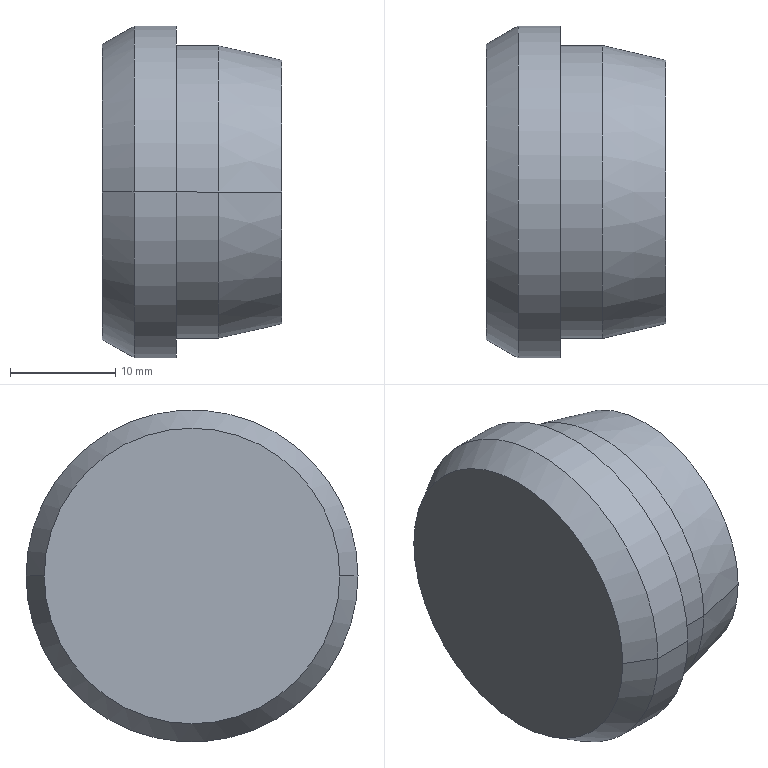Part | STEP file | DCV-000-041 | 1 solid | 11 faces | box 17 x 31.5 x 31.5 mm | volume 10923 mm3 | cone 4 | cylinder 4 | plane 3 | commonest cylinder face diameters 27.8 x2 31.5 x2
STEP:
#1=CARTESIAN_POINT('',(0.,0.,0.));
#2=DIRECTION('',(0.,0.,1.));
#3=DIRECTION('',(1.,0.,0.));
#4=AXIS2_PLACEMENT_3D('',#1,#2,#3);
#5=CARTESIAN_POINT('',(0.,14.018,0.));
#6=VERTEX_POINT('',#5);
#7=CARTESIAN_POINT('',(0.,-14.018,0.));
#8=VERTEX_POINT('',#7);
#9=CARTESIAN_POINT('',(0.,0.,0.));
#10=DIRECTION('',(1.,0.,0.));
#11=DIRECTION('',(0.,0.,-1.));
#12=AXIS2_PLACEMENT_3D('',#9,#10,#11);
#13=CIRCLE('',#12,14.018);
#14=CARTESIAN_POINT('',(1.5,0.,0.));
#15=DIRECTION('',(1.,0.,0.));
#16=DIRECTION('',(0.,1.,0.));
#17=AXIS2_PLACEMENT_3D('',#14,#15,#16);
#18=CONICAL_SURFACE('',#17,14.884,0.5236);
#19=CARTESIAN_POINT('',(-1.571,-1.5));
#20=DIRECTION('',(1.,0.));
#21=VECTOR('',#20,1.);
#22=LINE('',#19,#21);
#23=(GEOMETRIC_REPRESENTATION_CONTEXT(2)PARAMETRIC_REPRESENTATION_CONTEXT()REPRESENTATION_CONTEXT('',''));
#24=DEFINITIONAL_REPRESENTATION('',(#22),#23);
#25=PCURVE('',#18,#24);
#26=CARTESIAN_POINT('',(0.,14.018,0.));
#27=DIRECTION('',(-1.,0.,0.));
#28=DIRECTION('',(0.,0.,1.));
#29=AXIS2_PLACEMENT_3D('',#26,#27,#28);
#30=PLANE('',#29);
#31=CARTESIAN_POINT('',(-14.018,-14.018));
#32=CARTESIAN_POINT('',(-14.018,10.262));
#33=CARTESIAN_POINT('',(7.009,-1.878));
#34=CARTESIAN_POINT('',(28.036,-14.018));
#35=CARTESIAN_POINT('',(7.009,-26.158));
#36=CARTESIAN_POINT('',(-14.018,-38.298));
#37=CARTESIAN_POINT('',(-14.018,-14.018));
#38=(BOUNDED_CURVE()B_SPLINE_CURVE(2,(#31,#32,#33,#34,#35,#36,#37),.UNSPECIFIED.,.T.,.F.)B_SPLINE_CURVE_WITH_KNOTS((1,2,2,2,2,1),(-2.094,0.,2.094,4.189,6.283,8.378),.UNSPECIFIED.)CURVE()GEOMETRIC_REPRESENTATION_ITEM()RATIONAL_B_SPLINE_CURVE((1.,0.5,1.,0.5,1.,0.5,1.))REPRESENTATION_ITEM(''));
#39=(GEOMETRIC_REPRESENTATION_CONTEXT(2)PARAMETRIC_REPRESENTATION_CONTEXT()REPRESENTATION_CONTEXT('',''));
#40=DEFINITIONAL_REPRESENTATION('',(#38),#39);
#41=PCURVE('',#30,#40);
#42=SURFACE_CURVE('',#13,(#25,#41),.PCURVE_S1.);
#43=EDGE_CURVE('',#6,#8,#42,.T.);
#44=ORIENTED_EDGE('',*,*,#43,.T.);
#45=CARTESIAN_POINT('',(3.,-15.75,0.));
#46=VERTEX_POINT('',#45);
#47=CARTESIAN_POINT('',(1.5,-14.884,0.));
#48=DIRECTION('',(0.866,-0.5,0.));
#49=VECTOR('',#48,1.);
#50=LINE('',#47,#49);
#51=CARTESIAN_POINT('',(3.142,0.));
#52=DIRECTION('',(0.,1.));
#53=VECTOR('',#52,1.);
#54=LINE('',#51,#53);
#55=(GEOMETRIC_REPRESENTATION_CONTEXT(2)PARAMETRIC_REPRESENTATION_CONTEXT()REPRESENTATION_CONTEXT('',''));
#56=DEFINITIONAL_REPRESENTATION('',(#54),#55);
#57=PCURVE('',#18,#56);
#58=CARTESIAN_POINT('',(1.5,0.,0.));
#59=DIRECTION('',(1.,0.,0.));
#60=DIRECTION('',(0.,1.,0.));
#61=AXIS2_PLACEMENT_3D('',#58,#59,#60);
#62=CONICAL_SURFACE('',#61,14.884,0.5236);
#63=CARTESIAN_POINT('',(3.142,0.));
#64=DIRECTION('',(0.,1.));
#65=VECTOR('',#64,1.);
#66=LINE('',#63,#65);
#67=(GEOMETRIC_REPRESENTATION_CONTEXT(2)PARAMETRIC_REPRESENTATION_CONTEXT()REPRESENTATION_CONTEXT('',''));
#68=DEFINITIONAL_REPRESENTATION('',(#66),#67);
#69=PCURVE('',#62,#68);
#70=SURFACE_CURVE('',#50,(#57,#69),.PCURVE_S1.);
#71=EDGE_CURVE('',#8,#46,#70,.T.);
#72=ORIENTED_EDGE('',*,*,#71,.T.);
#73=CARTESIAN_POINT('',(3.,15.75,0.));
#74=VERTEX_POINT('',#73);
#75=CARTESIAN_POINT('',(3.,0.,0.));
#76=DIRECTION('',(1.,0.,0.));
#77=DIRECTION('',(0.,0.,-1.));
#78=AXIS2_PLACEMENT_3D('',#75,#76,#77);
#79=CIRCLE('',#78,15.75);
#80=CARTESIAN_POINT('',(-1.571,1.5));
#81=DIRECTION('',(1.,0.));
#82=VECTOR('',#81,1.);
#83=LINE('',#80,#82);
#84=(GEOMETRIC_REPRESENTATION_CONTEXT(2)PARAMETRIC_REPRESENTATION_CONTEXT()REPRESENTATION_CONTEXT('',''));
#85=DEFINITIONAL_REPRESENTATION('',(#83),#84);
#86=PCURVE('',#18,#85);
#87=CARTESIAN_POINT('',(5.,0.,0.));
#88=DIRECTION('',(1.,0.,0.));
#89=DIRECTION('',(0.,1.,0.));
#90=AXIS2_PLACEMENT_3D('',#87,#88,#89);
#91=CYLINDRICAL_SURFACE('',#90,15.75);
#92=CARTESIAN_POINT('',(-1.571,-2.));
#93=DIRECTION('',(1.,0.));
#94=VECTOR('',#93,1.);
#95=LINE('',#92,#94);
#96=(GEOMETRIC_REPRESENTATION_CONTEXT(2)PARAMETRIC_REPRESENTATION_CONTEXT()REPRESENTATION_CONTEXT('',''));
#97=DEFINITIONAL_REPRESENTATION('',(#95),#96);
#98=PCURVE('',#91,#97);
#99=SURFACE_CURVE('',#79,(#86,#98),.PCURVE_S1.);
#100=EDGE_CURVE('',#74,#46,#99,.T.);
#101=ORIENTED_EDGE('',*,*,#100,.F.);
#102=CARTESIAN_POINT('',(1.5,14.884,0.));
#103=DIRECTION('',(0.866,0.5,0.));
#104=VECTOR('',#103,1.);
#105=LINE('',#102,#104);
#106=CARTESIAN_POINT('',(0.,0.));
#107=DIRECTION('',(0.,1.));
#108=VECTOR('',#107,1.);
#109=LINE('',#106,#108);
#110=(GEOMETRIC_REPRESENTATION_CONTEXT(2)PARAMETRIC_REPRESENTATION_CONTEXT()REPRESENTATION_CONTEXT('',''));
#111=DEFINITIONAL_REPRESENTATION('',(#109),#110);
#112=PCURVE('',#18,#111);
#113=CARTESIAN_POINT('',(6.283,0.));
#114=DIRECTION('',(0.,1.));
#115=VECTOR('',#114,1.);
#116=LINE('',#113,#115);
#117=(GEOMETRIC_REPRESENTATION_CONTEXT(2)PARAMETRIC_REPRESENTATION_CONTEXT()REPRESENTATION_CONTEXT('',''));
#118=DEFINITIONAL_REPRESENTATION('',(#116),#117);
#119=PCURVE('',#62,#118);
#120=SURFACE_CURVE('',#105,(#112,#119),.PCURVE_S1.);
#121=EDGE_CURVE('',#6,#74,#120,.T.);
#122=ORIENTED_EDGE('',*,*,#121,.F.);
#123=EDGE_LOOP('',(#44,#72,#101,#122));
#124=FACE_BOUND('',#123,.T.);
#125=ADVANCED_FACE('',(#124),#18,.T.);
#126=ORIENTED_EDGE('',*,*,#100,.T.);
#127=CARTESIAN_POINT('',(7.,-15.75,0.));
#128=VERTEX_POINT('',#127);
#129=CARTESIAN_POINT('',(5.,-15.75,0.));
#130=DIRECTION('',(1.,0.,0.));
#131=VECTOR('',#130,1.);
#132=LINE('',#129,#131);
#133=CARTESIAN_POINT('',(3.142,0.));
#134=DIRECTION('',(0.,1.));
#135=VECTOR('',#134,1.);
#136=LINE('',#133,#135);
#137=(GEOMETRIC_REPRESENTATION_CONTEXT(2)PARAMETRIC_REPRESENTATION_CONTEXT()REPRESENTATION_CONTEXT('',''));
#138=DEFINITIONAL_REPRESENTATION('',(#136),#137);
#139=PCURVE('',#91,#138);
#140=CARTESIAN_POINT('',(5.,0.,0.));
#141=DIRECTION('',(1.,0.,0.));
#142=DIRECTION('',(0.,1.,0.));
#143=AXIS2_PLACEMENT_3D('',#140,#141,#142);
#144=CYLINDRICAL_SURFACE('',#143,15.75);
#145=CARTESIAN_POINT('',(3.142,0.));
#146=DIRECTION('',(0.,1.));
#147=VECTOR('',#146,1.);
#148=LINE('',#145,#147);
#149=(GEOMETRIC_REPRESENTATION_CONTEXT(2)PARAMETRIC_REPRESENTATION_CONTEXT()REPRESENTATION_CONTEXT('',''));
#150=DEFINITIONAL_REPRESENTATION('',(#148),#149);
#151=PCURVE('',#144,#150);
#152=SURFACE_CURVE('',#132,(#139,#151),.PCURVE_S1.);
#153=EDGE_CURVE('',#46,#128,#152,.T.);
#154=ORIENTED_EDGE('',*,*,#153,.T.);
#155=CARTESIAN_POINT('',(7.,15.75,0.));
#156=VERTEX_POINT('',#155);
#157=CARTESIAN_POINT('',(7.,0.,0.));
#158=DIRECTION('',(1.,0.,0.));
#159=DIRECTION('',(0.,0.,-1.));
#160=AXIS2_PLACEMENT_3D('',#157,#158,#159);
#161=CIRCLE('',#160,15.75);
#162=CARTESIAN_POINT('',(-1.571,2.));
#163=DIRECTION('',(1.,0.));
#164=VECTOR('',#163,1.);
#165=LINE('',#162,#164);
#166=(GEOMETRIC_REPRESENTATION_CONTEXT(2)PARAMETRIC_REPRESENTATION_CONTEXT()REPRESENTATION_CONTEXT('',''));
#167=DEFINITIONAL_REPRESENTATION('',(#165),#166);
#168=PCURVE('',#91,#167);
#169=CARTESIAN_POINT('',(7.,13.9,0.));
#170=DIRECTION('',(1.,0.,0.));
#171=DIRECTION('',(0.,-1.,0.));
#172=AXIS2_PLACEMENT_3D('',#169,#170,#171);
#173=PLANE('',#172);
#174=CARTESIAN_POINT('',(13.9,0.));
#175=DIRECTION('',(0.,1.));
#176=AXIS2_PLACEMENT_2D('',#174,#175);
#177=CIRCLE('',#176,15.75);
#178=(GEOMETRIC_REPRESENTATION_CONTEXT(2)PARAMETRIC_REPRESENTATION_CONTEXT()REPRESENTATION_CONTEXT('',''));
#179=DEFINITIONAL_REPRESENTATION('',(#177),#178);
#180=PCURVE('',#173,#179);
#181=SURFACE_CURVE('',#161,(#168,#180),.PCURVE_S1.);
#182=EDGE_CURVE('',#156,#128,#181,.T.);
#183=ORIENTED_EDGE('',*,*,#182,.F.);
#184=CARTESIAN_POINT('',(5.,15.75,0.));
#185=DIRECTION('',(1.,0.,0.));
#186=VECTOR('',#185,1.);
#187=LINE('',#184,#186);
#188=CARTESIAN_POINT('',(0.,0.));
#189=DIRECTION('',(0.,1.));
#190=VECTOR('',#189,1.);
#191=LINE('',#188,#190);
#192=(GEOMETRIC_REPRESENTATION_CONTEXT(2)PARAMETRIC_REPRESENTATION_CONTEXT()REPRESENTATION_CONTEXT('',''));
#193=DEFINITIONAL_REPRESENTATION('',(#191),#192);
#194=PCURVE('',#91,#193);
#195=CARTESIAN_POINT('',(6.283,0.));
#196=DIRECTION('',(0.,1.));
#197=VECTOR('',#196,1.);
#198=LINE('',#195,#197);
#199=(GEOMETRIC_REPRESENTATION_CONTEXT(2)PARAMETRIC_REPRESENTATION_CONTEXT()REPRESENTATION_CONTEXT('',''));
#200=DEFINITIONAL_REPRESENTATION('',(#198),#199);
#201=PCURVE('',#144,#200);
#202=SURFACE_CURVE('',#187,(#194,#201),.PCURVE_S1.);
#203=EDGE_CURVE('',#74,#156,#202,.T.);
#204=ORIENTED_EDGE('',*,*,#203,.F.);
#205=EDGE_LOOP('',(#126,#154,#183,#204));
#206=FACE_BOUND('',#205,.T.);
#207=ADVANCED_FACE('',(#206),#91,.T.);
#208=CARTESIAN_POINT('',(7.,13.9,0.));
#209=VERTEX_POINT('',#208);
#210=CARTESIAN_POINT('',(7.,-13.9,0.));
#211=VERTEX_POINT('',#210);
#212=CARTESIAN_POINT('',(7.,0.,0.));
#213=DIRECTION('',(1.,0.,0.));
#214=DIRECTION('',(0.,0.,-1.));
#215=AXIS2_PLACEMENT_3D('',#212,#213,#214);
#216=CIRCLE('',#215,13.9);
#217=CARTESIAN_POINT('',(9.,0.,0.));
#218=DIRECTION('',(1.,0.,0.));
#219=DIRECTION('',(0.,1.,0.));
#220=AXIS2_PLACEMENT_3D('',#217,#218,#219);
#221=CYLINDRICAL_SURFACE('',#220,13.9);
#222=CARTESIAN_POINT('',(-1.571,-2.));
#223=DIRECTION('',(1.,0.));
#224=VECTOR('',#223,1.);
#225=LINE('',#222,#224);
#226=(GEOMETRIC_REPRESENTATION_CONTEXT(2)PARAMETRIC_REPRESENTATION_CONTEXT()REPRESENTATION_CONTEXT('',''));
#227=DEFINITIONAL_REPRESENTATION('',(#225),#226);
#228=PCURVE('',#221,#227);
#229=CARTESIAN_POINT('',(13.9,0.));
#230=DIRECTION('',(0.,1.));
#231=AXIS2_PLACEMENT_2D('',#229,#230);
#232=CIRCLE('',#231,13.9);
#233=(GEOMETRIC_REPRESENTATION_CONTEXT(2)PARAMETRIC_REPRESENTATION_CONTEXT()REPRESENTATION_CONTEXT('',''));
#234=DEFINITIONAL_REPRESENTATION('',(#232),#233);
#235=PCURVE('',#173,#234);
#236=SURFACE_CURVE('',#216,(#228,#235),.PCURVE_S1.);
#237=EDGE_CURVE('',#209,#211,#236,.T.);
#238=ORIENTED_EDGE('',*,*,#237,.T.);
#239=CARTESIAN_POINT('',(11.,-13.9,0.));
#240=VERTEX_POINT('',#239);
#241=CARTESIAN_POINT('',(9.,-13.9,0.));
#242=DIRECTION('',(1.,0.,0.));
#243=VECTOR('',#242,1.);
#244=LINE('',#241,#243);
#245=CARTESIAN_POINT('',(3.142,0.));
#246=DIRECTION('',(0.,1.));
#247=VECTOR('',#246,1.);
#248=LINE('',#245,#247);
#249=(GEOMETRIC_REPRESENTATION_CONTEXT(2)PARAMETRIC_REPRESENTATION_CONTEXT()REPRESENTATION_CONTEXT('',''));
#250=DEFINITIONAL_REPRESENTATION('',(#248),#249);
#251=PCURVE('',#221,#250);
#252=CARTESIAN_POINT('',(9.,0.,0.));
#253=DIRECTION('',(1.,0.,0.));
#254=DIRECTION('',(0.,1.,0.));
#255=AXIS2_PLACEMENT_3D('',#252,#253,#254);
#256=CYLINDRICAL_SURFACE('',#255,13.9);
#257=CARTESIAN_POINT('',(3.142,0.));
#258=DIRECTION('',(0.,1.));
#259=VECTOR('',#258,1.);
#260=LINE('',#257,#259);
#261=(GEOMETRIC_REPRESENTATION_CONTEXT(2)PARAMETRIC_REPRESENTATION_CONTEXT()REPRESENTATION_CONTEXT('',''));
#262=DEFINITIONAL_REPRESENTATION('',(#260),#261);
#263=PCURVE('',#256,#262);
#264=SURFACE_CURVE('',#244,(#251,#263),.PCURVE_S1.);
#265=EDGE_CURVE('',#211,#240,#264,.T.);
#266=ORIENTED_EDGE('',*,*,#265,.T.);
#267=CARTESIAN_POINT('',(11.,13.9,0.));
#268=VERTEX_POINT('',#267);
#269=CARTESIAN_POINT('',(11.,0.,0.));
#270=DIRECTION('',(1.,0.,0.));
#271=DIRECTION('',(0.,0.,-1.));
#272=AXIS2_PLACEMENT_3D('',#269,#270,#271);
#273=CIRCLE('',#272,13.9);
#274=CARTESIAN_POINT('',(-1.571,2.));
#275=DIRECTION('',(1.,0.));
#276=VECTOR('',#275,1.);
#277=LINE('',#274,#276);
#278=(GEOMETRIC_REPRESENTATION_CONTEXT(2)PARAMETRIC_REPRESENTATION_CONTEXT()REPRESENTATION_CONTEXT('',''));
#279=DEFINITIONAL_REPRESENTATION('',(#277),#278);
#280=PCURVE('',#221,#279);
#281=CARTESIAN_POINT('',(14.,0.,0.));
#282=DIRECTION('',(-1.,0.,0.));
#283=DIRECTION('',(0.,1.,0.));
#284=AXIS2_PLACEMENT_3D('',#281,#282,#283);
#285=CONICAL_SURFACE('',#284,13.2,0.2292);
#286=CARTESIAN_POINT('',(7.854,3.));
#287=DIRECTION('',(-1.,0.));
#288=VECTOR('',#287,1.);
#289=LINE('',#286,#288);
#290=(GEOMETRIC_REPRESENTATION_CONTEXT(2)PARAMETRIC_REPRESENTATION_CONTEXT()REPRESENTATION_CONTEXT('',''));
#291=DEFINITIONAL_REPRESENTATION('',(#289),#290);
#292=PCURVE('',#285,#291);
#293=SURFACE_CURVE('',#273,(#280,#292),.PCURVE_S1.);
#294=EDGE_CURVE('',#268,#240,#293,.T.);
#295=ORIENTED_EDGE('',*,*,#294,.F.);
#296=CARTESIAN_POINT('',(9.,13.9,0.));
#297=DIRECTION('',(1.,0.,0.));
#298=VECTOR('',#297,1.);
#299=LINE('',#296,#298);
#300=CARTESIAN_POINT('',(0.,0.));
#301=DIRECTION('',(0.,1.));
#302=VECTOR('',#301,1.);
#303=LINE('',#300,#302);
#304=(GEOMETRIC_REPRESENTATION_CONTEXT(2)PARAMETRIC_REPRESENTATION_CONTEXT()REPRESENTATION_CONTEXT('',''));
#305=DEFINITIONAL_REPRESENTATION('',(#303),#304);
#306=PCURVE('',#221,#305);
#307=CARTESIAN_POINT('',(6.283,0.));
#308=DIRECTION('',(0.,1.));
#309=VECTOR('',#308,1.);
#310=LINE('',#307,#309);
#311=(GEOMETRIC_REPRESENTATION_CONTEXT(2)PARAMETRIC_REPRESENTATION_CONTEXT()REPRESENTATION_CONTEXT('',''));
#312=DEFINITIONAL_REPRESENTATION('',(#310),#311);
#313=PCURVE('',#256,#312);
#314=SURFACE_CURVE('',#299,(#306,#313),.PCURVE_S1.);
#315=EDGE_CURVE('',#209,#268,#314,.T.);
#316=ORIENTED_EDGE('',*,*,#315,.F.);
#317=EDGE_LOOP('',(#238,#266,#295,#316));
#318=FACE_BOUND('',#317,.T.);
#319=ADVANCED_FACE('',(#318),#221,.T.);
#320=CARTESIAN_POINT('',(17.,-12.5,0.));
#321=VERTEX_POINT('',#320);
#322=CARTESIAN_POINT('',(17.,12.5,0.));
#323=VERTEX_POINT('',#322);
#324=CARTESIAN_POINT('',(17.,0.,0.));
#325=DIRECTION('',(1.,0.,0.));
#326=DIRECTION('',(0.,0.,-1.));
#327=AXIS2_PLACEMENT_3D('',#324,#325,#326);
#328=CIRCLE('',#327,12.5);
#329=CARTESIAN_POINT('',(14.,0.,0.));
#330=DIRECTION('',(-1.,0.,0.));
#331=DIRECTION('',(0.,1.,0.));
#332=AXIS2_PLACEMENT_3D('',#329,#330,#331);
#333=CONICAL_SURFACE('',#332,13.2,0.2292);
#334=CARTESIAN_POINT('',(7.854,-3.));
#335=DIRECTION('',(-1.,0.));
#336=VECTOR('',#335,1.);
#337=LINE('',#334,#336);
#338=(GEOMETRIC_REPRESENTATION_CONTEXT(2)PARAMETRIC_REPRESENTATION_CONTEXT()REPRESENTATION_CONTEXT('',''));
#339=DEFINITIONAL_REPRESENTATION('',(#337),#338);
#340=PCURVE('',#333,#339);
#341=CARTESIAN_POINT('',(17.,0.,0.));
#342=DIRECTION('',(1.,0.,0.));
#343=DIRECTION('',(0.,-1.,0.));
#344=AXIS2_PLACEMENT_3D('',#341,#342,#343);
#345=PLANE('',#344);
#346=CARTESIAN_POINT('',(0.,0.));
#347=DIRECTION('',(0.,1.));
#348=AXIS2_PLACEMENT_2D('',#346,#347);
#349=CIRCLE('',#348,12.5);
#350=(GEOMETRIC_REPRESENTATION_CONTEXT(2)PARAMETRIC_REPRESENTATION_CONTEXT()REPRESENTATION_CONTEXT('',''));
#351=DEFINITIONAL_REPRESENTATION('',(#349),#350);
#352=PCURVE('',#345,#351);
#353=SURFACE_CURVE('',#328,(#340,#352),.PCURVE_S1.);
#354=EDGE_CURVE('',#321,#323,#353,.T.);
#355=ORIENTED_EDGE('',*,*,#354,.F.);
#356=CARTESIAN_POINT('',(14.,-13.2,0.));
#357=DIRECTION('',(-0.9738,-0.2272,0.));
#358=VECTOR('',#357,1.);
#359=LINE('',#356,#358);
#360=CARTESIAN_POINT('',(3.142,0.));
#361=DIRECTION('',(0.,1.));
#362=VECTOR('',#361,1.);
#363=LINE('',#360,#362);
#364=(GEOMETRIC_REPRESENTATION_CONTEXT(2)PARAMETRIC_REPRESENTATION_CONTEXT()REPRESENTATION_CONTEXT('',''));
#365=DEFINITIONAL_REPRESENTATION('',(#363),#364);
#366=PCURVE('',#333,#365);
#367=CARTESIAN_POINT('',(3.142,0.));
#368=DIRECTION('',(0.,1.));
#369=VECTOR('',#368,1.);
#370=LINE('',#367,#369);
#371=(GEOMETRIC_REPRESENTATION_CONTEXT(2)PARAMETRIC_REPRESENTATION_CONTEXT()REPRESENTATION_CONTEXT('',''));
#372=DEFINITIONAL_REPRESENTATION('',(#370),#371);
#373=PCURVE('',#285,#372);
#374=SURFACE_CURVE('',#359,(#366,#373),.PCURVE_S1.);
#375=EDGE_CURVE('',#321,#240,#374,.T.);
#376=ORIENTED_EDGE('',*,*,#375,.T.);
#377=CARTESIAN_POINT('',(11.,0.,0.));
#378=DIRECTION('',(1.,0.,0.));
#379=DIRECTION('',(0.,0.,-1.));
#380=AXIS2_PLACEMENT_3D('',#377,#378,#379);
#381=CIRCLE('',#380,13.9);
#382=CARTESIAN_POINT('',(7.854,3.));
#383=DIRECTION('',(-1.,0.));
#384=VECTOR('',#383,1.);
#385=LINE('',#382,#384);
#386=(GEOMETRIC_REPRESENTATION_CONTEXT(2)PARAMETRIC_REPRESENTATION_CONTEXT()REPRESENTATION_CONTEXT('',''));
#387=DEFINITIONAL_REPRESENTATION('',(#385),#386);
#388=PCURVE('',#333,#387);
#389=CARTESIAN_POINT('',(-1.571,2.));
#390=DIRECTION('',(1.,0.));
#391=VECTOR('',#390,1.);
#392=LINE('',#389,#391);
#393=(GEOMETRIC_REPRESENTATION_CONTEXT(2)PARAMETRIC_REPRESENTATION_CONTEXT()REPRESENTATION_CONTEXT('',''));
#394=DEFINITIONAL_REPRESENTATION('',(#392),#393);
#395=PCURVE('',#256,#394);
#396=SURFACE_CURVE('',#381,(#388,#395),.PCURVE_S1.);
#397=EDGE_CURVE('',#240,#268,#396,.T.);
#398=ORIENTED_EDGE('',*,*,#397,.T.);
#399=CARTESIAN_POINT('',(14.,13.2,0.));
#400=DIRECTION('',(-0.9738,0.2272,0.));
#401=VECTOR('',#400,1.);
#402=LINE('',#399,#401);
#403=CARTESIAN_POINT('',(0.,0.));
#404=DIRECTION('',(0.,1.));
#405=VECTOR('',#404,1.);
#406=LINE('',#403,#405);
#407=(GEOMETRIC_REPRESENTATION_CONTEXT(2)PARAMETRIC_REPRESENTATION_CONTEXT()REPRESENTATION_CONTEXT('',''));
#408=DEFINITIONAL_REPRESENTATION('',(#406),#407);
#409=PCURVE('',#333,#408);
#410=CARTESIAN_POINT('',(6.283,0.));
#411=DIRECTION('',(0.,1.));
#412=VECTOR('',#411,1.);
#413=LINE('',#410,#412);
#414=(GEOMETRIC_REPRESENTATION_CONTEXT(2)PARAMETRIC_REPRESENTATION_CONTEXT()REPRESENTATION_CONTEXT('',''));
#415=DEFINITIONAL_REPRESENTATION('',(#413),#414);
#416=PCURVE('',#285,#415);
#417=SURFACE_CURVE('',#402,(#409,#416),.PCURVE_S1.);
#418=EDGE_CURVE('',#323,#268,#417,.T.);
#419=ORIENTED_EDGE('',*,*,#418,.F.);
#420=EDGE_LOOP('',(#355,#376,#398,#419));
#421=FACE_BOUND('',#420,.T.);
#422=ADVANCED_FACE('',(#421),#333,.T.);
#423=CARTESIAN_POINT('',(17.,0.,0.));
#424=DIRECTION('',(1.,0.,0.));
#425=DIRECTION('',(0.,0.,-1.));
#426=AXIS2_PLACEMENT_3D('',#423,#424,#425);
#427=CIRCLE('',#426,12.5);
#428=CARTESIAN_POINT('',(0.,0.));
#429=DIRECTION('',(0.,1.));
#430=AXIS2_PLACEMENT_2D('',#428,#429);
#431=CIRCLE('',#430,12.5);
#432=(GEOMETRIC_REPRESENTATION_CONTEXT(2)PARAMETRIC_REPRESENTATION_CONTEXT()REPRESENTATION_CONTEXT('',''));
#433=DEFINITIONAL_REPRESENTATION('',(#431),#432);
#434=PCURVE('',#345,#433);
#435=CARTESIAN_POINT('',(7.854,-3.));
#436=DIRECTION('',(-1.,0.));
#437=VECTOR('',#436,1.);
#438=LINE('',#435,#437);
#439=(GEOMETRIC_REPRESENTATION_CONTEXT(2)PARAMETRIC_REPRESENTATION_CONTEXT()REPRESENTATION_CONTEXT('',''));
#440=DEFINITIONAL_REPRESENTATION('',(#438),#439);
#441=PCURVE('',#285,#440);
#442=SURFACE_CURVE('',#427,(#434,#441),.PCURVE_S1.);
#443=EDGE_CURVE('',#323,#321,#442,.T.);
#444=ORIENTED_EDGE('',*,*,#443,.T.);
#445=ORIENTED_EDGE('',*,*,#354,.T.);
#446=EDGE_LOOP('',(#444,#445));
#447=FACE_BOUND('',#446,.T.);
#448=ADVANCED_FACE('',(#447),#345,.T.);
#449=ORIENTED_EDGE('',*,*,#375,.F.);
#450=ORIENTED_EDGE('',*,*,#443,.F.);
#451=ORIENTED_EDGE('',*,*,#418,.T.);
#452=ORIENTED_EDGE('',*,*,#294,.T.);
#453=EDGE_LOOP('',(#449,#450,#451,#452));
#454=FACE_BOUND('',#453,.T.);
#455=ADVANCED_FACE('',(#454),#285,.T.);
#456=ORIENTED_EDGE('',*,*,#265,.F.);
#457=CARTESIAN_POINT('',(7.,0.,0.));
#458=DIRECTION('',(1.,0.,0.));
#459=DIRECTION('',(0.,0.,-1.));
#460=AXIS2_PLACEMENT_3D('',#457,#458,#459);
#461=CIRCLE('',#460,13.9);
#462=CARTESIAN_POINT('',(-1.571,-2.));
#463=DIRECTION('',(1.,0.));
#464=VECTOR('',#463,1.);
#465=LINE('',#462,#464);
#466=(GEOMETRIC_REPRESENTATION_CONTEXT(2)PARAMETRIC_REPRESENTATION_CONTEXT()REPRESENTATION_CONTEXT('',''));
#467=DEFINITIONAL_REPRESENTATION('',(#465),#466);
#468=PCURVE('',#256,#467);
#469=CARTESIAN_POINT('',(13.9,0.));
#470=DIRECTION('',(0.,1.));
#471=AXIS2_PLACEMENT_2D('',#469,#470);
#472=CIRCLE('',#471,13.9);
#473=(GEOMETRIC_REPRESENTATION_CONTEXT(2)PARAMETRIC_REPRESENTATION_CONTEXT()REPRESENTATION_CONTEXT('',''));
#474=DEFINITIONAL_REPRESENTATION('',(#472),#473);
#475=PCURVE('',#173,#474);
#476=SURFACE_CURVE('',#461,(#468,#475),.PCURVE_S1.);
#477=EDGE_CURVE('',#211,#209,#476,.T.);
#478=ORIENTED_EDGE('',*,*,#477,.T.);
#479=ORIENTED_EDGE('',*,*,#315,.T.);
#480=ORIENTED_EDGE('',*,*,#397,.F.);
#481=EDGE_LOOP('',(#456,#478,#479,#480));
#482=FACE_BOUND('',#481,.T.);
#483=ADVANCED_FACE('',(#482),#256,.T.);
#484=ORIENTED_EDGE('',*,*,#237,.F.);
#485=ORIENTED_EDGE('',*,*,#477,.F.);
#486=EDGE_LOOP('',(#484,#485));
#487=FACE_BOUND('',#486,.T.);
#488=ORIENTED_EDGE('',*,*,#182,.T.);
#489=CARTESIAN_POINT('',(7.,0.,0.));
#490=DIRECTION('',(1.,0.,0.));
#491=DIRECTION('',(0.,0.,-1.));
#492=AXIS2_PLACEMENT_3D('',#489,#490,#491);
#493=CIRCLE('',#492,15.75);
#494=CARTESIAN_POINT('',(13.9,0.));
#495=DIRECTION('',(0.,1.));
#496=AXIS2_PLACEMENT_2D('',#494,#495);
#497=CIRCLE('',#496,15.75);
#498=(GEOMETRIC_REPRESENTATION_CONTEXT(2)PARAMETRIC_REPRESENTATION_CONTEXT()REPRESENTATION_CONTEXT('',''));
#499=DEFINITIONAL_REPRESENTATION('',(#497),#498);
#500=PCURVE('',#173,#499);
#501=CARTESIAN_POINT('',(-1.571,2.));
#502=DIRECTION('',(1.,0.));
#503=VECTOR('',#502,1.);
#504=LINE('',#501,#503);
#505=(GEOMETRIC_REPRESENTATION_CONTEXT(2)PARAMETRIC_REPRESENTATION_CONTEXT()REPRESENTATION_CONTEXT('',''));
#506=DEFINITIONAL_REPRESENTATION('',(#504),#505);
#507=PCURVE('',#144,#506);
#508=SURFACE_CURVE('',#493,(#500,#507),.PCURVE_S1.);
#509=EDGE_CURVE('',#128,#156,#508,.T.);
#510=ORIENTED_EDGE('',*,*,#509,.T.);
#511=EDGE_LOOP('',(#488,#510));
#512=FACE_BOUND('',#511,.T.);
#513=ADVANCED_FACE('',(#487,#512),#173,.T.);
#514=ORIENTED_EDGE('',*,*,#153,.F.);
#515=CARTESIAN_POINT('',(3.,0.,0.));
#516=DIRECTION('',(1.,0.,0.));
#517=DIRECTION('',(0.,0.,-1.));
#518=AXIS2_PLACEMENT_3D('',#515,#516,#517);
#519=CIRCLE('',#518,15.75);
#520=CARTESIAN_POINT('',(-1.571,-2.));
#521=DIRECTION('',(1.,0.));
#522=VECTOR('',#521,1.);
#523=LINE('',#520,#522);
#524=(GEOMETRIC_REPRESENTATION_CONTEXT(2)PARAMETRIC_REPRESENTATION_CONTEXT()REPRESENTATION_CONTEXT('',''));
#525=DEFINITIONAL_REPRESENTATION('',(#523),#524);
#526=PCURVE('',#144,#525);
#527=CARTESIAN_POINT('',(-1.571,1.5));
#528=DIRECTION('',(1.,0.));
#529=VECTOR('',#528,1.);
#530=LINE('',#527,#529);
#531=(GEOMETRIC_REPRESENTATION_CONTEXT(2)PARAMETRIC_REPRESENTATION_CONTEXT()REPRESENTATION_CONTEXT('',''));
#532=DEFINITIONAL_REPRESENTATION('',(#530),#531);
#533=PCURVE('',#62,#532);
#534=SURFACE_CURVE('',#519,(#526,#533),.PCURVE_S1.);
#535=EDGE_CURVE('',#46,#74,#534,.T.);
#536=ORIENTED_EDGE('',*,*,#535,.T.);
#537=ORIENTED_EDGE('',*,*,#203,.T.);
#538=ORIENTED_EDGE('',*,*,#509,.F.);
#539=EDGE_LOOP('',(#514,#536,#537,#538));
#540=FACE_BOUND('',#539,.T.);
#541=ADVANCED_FACE('',(#540),#144,.T.);
#542=ORIENTED_EDGE('',*,*,#71,.F.);
#543=CARTESIAN_POINT('',(0.,0.,0.));
#544=DIRECTION('',(1.,0.,0.));
#545=DIRECTION('',(0.,0.,-1.));
#546=AXIS2_PLACEMENT_3D('',#543,#544,#545);
#547=CIRCLE('',#546,14.018);
#548=CARTESIAN_POINT('',(-1.571,-1.5));
#549=DIRECTION('',(1.,0.));
#550=VECTOR('',#549,1.);
#551=LINE('',#548,#550);
#552=(GEOMETRIC_REPRESENTATION_CONTEXT(2)PARAMETRIC_REPRESENTATION_CONTEXT()REPRESENTATION_CONTEXT('',''));
#553=DEFINITIONAL_REPRESENTATION('',(#551),#552);
#554=PCURVE('',#62,#553);
#555=CARTESIAN_POINT('',(-14.018,-14.018));
#556=CARTESIAN_POINT('',(-14.018,10.262));
#557=CARTESIAN_POINT('',(7.009,-1.878));
#558=CARTESIAN_POINT('',(28.036,-14.018));
#559=CARTESIAN_POINT('',(7.009,-26.158));
#560=CARTESIAN_POINT('',(-14.018,-38.298));
#561=CARTESIAN_POINT('',(-14.018,-14.018));
#562=(BOUNDED_CURVE()B_SPLINE_CURVE(2,(#555,#556,#557,#558,#559,#560,#561),.UNSPECIFIED.,.T.,.F.)B_SPLINE_CURVE_WITH_KNOTS((1,2,2,2,2,1),(-2.094,0.,2.094,4.189,6.283,8.378),.UNSPECIFIED.)CURVE()GEOMETRIC_REPRESENTATION_ITEM()RATIONAL_B_SPLINE_CURVE((1.,0.5,1.,0.5,1.,0.5,1.))REPRESENTATION_ITEM(''));
#563=(GEOMETRIC_REPRESENTATION_CONTEXT(2)PARAMETRIC_REPRESENTATION_CONTEXT()REPRESENTATION_CONTEXT('',''));
#564=DEFINITIONAL_REPRESENTATION('',(#562),#563);
#565=PCURVE('',#30,#564);
#566=SURFACE_CURVE('',#547,(#554,#565),.PCURVE_S1.);
#567=EDGE_CURVE('',#8,#6,#566,.T.);
#568=ORIENTED_EDGE('',*,*,#567,.T.);
#569=ORIENTED_EDGE('',*,*,#121,.T.);
#570=ORIENTED_EDGE('',*,*,#535,.F.);
#571=EDGE_LOOP('',(#542,#568,#569,#570));
#572=FACE_BOUND('',#571,.T.);
#573=ADVANCED_FACE('',(#572),#62,.T.);
#574=ORIENTED_EDGE('',*,*,#43,.F.);
#575=ORIENTED_EDGE('',*,*,#567,.F.);
#576=EDGE_LOOP('',(#574,#575));
#577=FACE_BOUND('',#576,.T.);
#578=ADVANCED_FACE('',(#577),#30,.T.);
#579=CLOSED_SHELL('',(#125,#207,#319,#422,#448,#455,#483,#513,#541,#573,#578));
#580=MANIFOLD_SOLID_BREP('',#579);
#581=(LENGTH_UNIT()NAMED_UNIT(*)SI_UNIT(.MILLI.,.METRE.));
#582=UNCERTAINTY_MEASURE_WITH_UNIT(LENGTH_MEASURE(0.0000001),#581,'','');
#583=(NAMED_UNIT(*)PLANE_ANGLE_UNIT()SI_UNIT($,.RADIAN.));
#584=(NAMED_UNIT(*)SI_UNIT($,.STERADIAN.)SOLID_ANGLE_UNIT());
#585=(GEOMETRIC_REPRESENTATION_CONTEXT(3)GLOBAL_UNCERTAINTY_ASSIGNED_CONTEXT((#582))GLOBAL_UNIT_ASSIGNED_CONTEXT((#581,#583,#584))REPRESENTATION_CONTEXT('',''));
#586=ADVANCED_BREP_SHAPE_REPRESENTATION('',(#4,#580),#585);